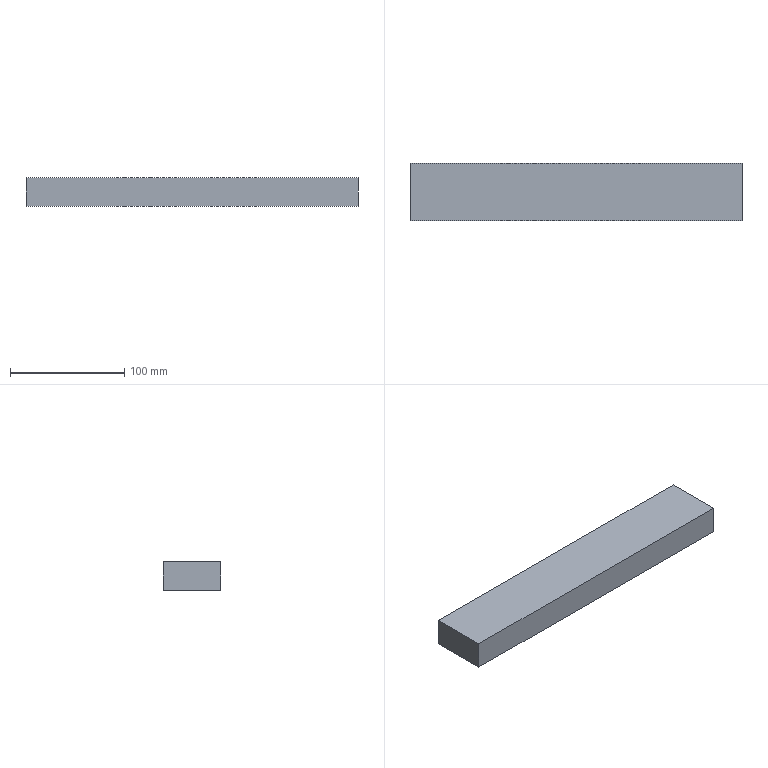Part | SolidWorks | features BaseBody 1 | 1 solid | 6 faces | box 290 x 50 x 25 mm | volume 362500 mm3 | plane 6
STEP:
#1=CARTESIAN_POINT('',(-145.,25.,0.));
#2=VERTEX_POINT('',#1);
#3=CARTESIAN_POINT('',(-145.,-25.,0.));
#4=VERTEX_POINT('',#3);
#5=CARTESIAN_POINT('',(-145.,-25.,0.));
#6=DIRECTION('',(0.,-1.,0.));
#7=VECTOR('',#6,1000.);
#8=LINE('',#5,#7);
#9=EDGE_CURVE('',#2,#4,#8,.T.);
#10=ORIENTED_EDGE('',*,*,#9,.T.);
#11=CARTESIAN_POINT('',(-145.,-25.,25.));
#12=VERTEX_POINT('',#11);
#13=CARTESIAN_POINT('',(-145.,-25.,25.));
#14=DIRECTION('',(0.,0.,-1.));
#15=VECTOR('',#14,1000.);
#16=LINE('',#13,#15);
#17=EDGE_CURVE('',#12,#4,#16,.T.);
#18=ORIENTED_EDGE('',*,*,#17,.F.);
#19=CARTESIAN_POINT('',(-145.,25.,25.));
#20=VERTEX_POINT('',#19);
#21=CARTESIAN_POINT('',(-145.,-25.,25.));
#22=DIRECTION('',(0.,-1.,0.));
#23=VECTOR('',#22,1000.);
#24=LINE('',#21,#23);
#25=EDGE_CURVE('',#20,#12,#24,.T.);
#26=ORIENTED_EDGE('',*,*,#25,.F.);
#27=CARTESIAN_POINT('',(-145.,25.,25.));
#28=DIRECTION('',(0.,0.,-1.));
#29=VECTOR('',#28,1000.);
#30=LINE('',#27,#29);
#31=EDGE_CURVE('',#20,#2,#30,.T.);
#32=ORIENTED_EDGE('',*,*,#31,.T.);
#33=EDGE_LOOP('',(#10,#18,#26,#32));
#34=FACE_OUTER_BOUND('',#33,.T.);
#35=CARTESIAN_POINT('',(-145.,-25.,25.));
#36=DIRECTION('',(1.,0.,0.));
#37=DIRECTION('',(0.,0.,-1.));
#38=AXIS2_PLACEMENT_3D('',#35,#36,#37);
#39=PLANE('',#38);
#40=ADVANCED_FACE('',(#34),#39,.F.);
#41=CARTESIAN_POINT('',(145.,-25.,0.));
#42=VERTEX_POINT('',#41);
#43=CARTESIAN_POINT('',(145.,-25.,0.));
#44=DIRECTION('',(1.,0.,0.));
#45=VECTOR('',#44,1000.);
#46=LINE('',#43,#45);
#47=EDGE_CURVE('',#4,#42,#46,.T.);
#48=ORIENTED_EDGE('',*,*,#47,.T.);
#49=CARTESIAN_POINT('',(145.,-25.,25.));
#50=VERTEX_POINT('',#49);
#51=CARTESIAN_POINT('',(145.,-25.,25.));
#52=DIRECTION('',(0.,0.,-1.));
#53=VECTOR('',#52,1000.);
#54=LINE('',#51,#53);
#55=EDGE_CURVE('',#50,#42,#54,.T.);
#56=ORIENTED_EDGE('',*,*,#55,.F.);
#57=CARTESIAN_POINT('',(145.,-25.,25.));
#58=DIRECTION('',(1.,0.,0.));
#59=VECTOR('',#58,1000.);
#60=LINE('',#57,#59);
#61=EDGE_CURVE('',#12,#50,#60,.T.);
#62=ORIENTED_EDGE('',*,*,#61,.F.);
#63=ORIENTED_EDGE('',*,*,#17,.T.);
#64=EDGE_LOOP('',(#48,#56,#62,#63));
#65=FACE_OUTER_BOUND('',#64,.T.);
#66=CARTESIAN_POINT('',(145.,-25.,25.));
#67=DIRECTION('',(0.,1.,0.));
#68=DIRECTION('',(-1.,0.,0.));
#69=AXIS2_PLACEMENT_3D('',#66,#67,#68);
#70=PLANE('',#69);
#71=ADVANCED_FACE('',(#65),#70,.F.);
#72=CARTESIAN_POINT('',(145.,25.,0.));
#73=VERTEX_POINT('',#72);
#74=CARTESIAN_POINT('',(145.,-25.,0.));
#75=DIRECTION('',(0.,1.,0.));
#76=VECTOR('',#75,1000.);
#77=LINE('',#74,#76);
#78=EDGE_CURVE('',#42,#73,#77,.T.);
#79=ORIENTED_EDGE('',*,*,#78,.T.);
#80=CARTESIAN_POINT('',(145.,25.,25.));
#81=VERTEX_POINT('',#80);
#82=CARTESIAN_POINT('',(145.,25.,25.));
#83=DIRECTION('',(0.,0.,-1.));
#84=VECTOR('',#83,1000.);
#85=LINE('',#82,#84);
#86=EDGE_CURVE('',#81,#73,#85,.T.);
#87=ORIENTED_EDGE('',*,*,#86,.F.);
#88=CARTESIAN_POINT('',(145.,-25.,25.));
#89=DIRECTION('',(0.,1.,0.));
#90=VECTOR('',#89,1000.);
#91=LINE('',#88,#90);
#92=EDGE_CURVE('',#50,#81,#91,.T.);
#93=ORIENTED_EDGE('',*,*,#92,.F.);
#94=ORIENTED_EDGE('',*,*,#55,.T.);
#95=EDGE_LOOP('',(#79,#87,#93,#94));
#96=FACE_OUTER_BOUND('',#95,.T.);
#97=CARTESIAN_POINT('',(145.,-25.,25.));
#98=DIRECTION('',(-1.,0.,0.));
#99=DIRECTION('',(0.,0.,1.));
#100=AXIS2_PLACEMENT_3D('',#97,#98,#99);
#101=PLANE('',#100);
#102=ADVANCED_FACE('',(#96),#101,.F.);
#103=CARTESIAN_POINT('',(145.,25.,0.));
#104=DIRECTION('',(-1.,0.,0.));
#105=VECTOR('',#104,1000.);
#106=LINE('',#103,#105);
#107=EDGE_CURVE('',#73,#2,#106,.T.);
#108=ORIENTED_EDGE('',*,*,#107,.T.);
#109=ORIENTED_EDGE('',*,*,#31,.F.);
#110=CARTESIAN_POINT('',(145.,25.,25.));
#111=DIRECTION('',(-1.,0.,0.));
#112=VECTOR('',#111,1000.);
#113=LINE('',#110,#112);
#114=EDGE_CURVE('',#81,#20,#113,.T.);
#115=ORIENTED_EDGE('',*,*,#114,.F.);
#116=ORIENTED_EDGE('',*,*,#86,.T.);
#117=EDGE_LOOP('',(#108,#109,#115,#116));
#118=FACE_OUTER_BOUND('',#117,.T.);
#119=CARTESIAN_POINT('',(145.,25.,25.));
#120=DIRECTION('',(0.,-1.,0.));
#121=DIRECTION('',(1.,0.,0.));
#122=AXIS2_PLACEMENT_3D('',#119,#120,#121);
#123=PLANE('',#122);
#124=ADVANCED_FACE('',(#118),#123,.F.);
#125=ORIENTED_EDGE('',*,*,#25,.T.);
#126=ORIENTED_EDGE('',*,*,#61,.T.);
#127=ORIENTED_EDGE('',*,*,#92,.T.);
#128=ORIENTED_EDGE('',*,*,#114,.T.);
#129=EDGE_LOOP('',(#125,#126,#127,#128));
#130=FACE_OUTER_BOUND('',#129,.T.);
#131=CARTESIAN_POINT('',(0.,0.,25.));
#132=DIRECTION('',(0.,0.,1.));
#133=DIRECTION('',(1.,0.,0.));
#134=AXIS2_PLACEMENT_3D('',#131,#132,#133);
#135=PLANE('',#134);
#136=ADVANCED_FACE('',(#130),#135,.T.);
#137=ORIENTED_EDGE('',*,*,#9,.F.);
#138=ORIENTED_EDGE('',*,*,#107,.F.);
#139=ORIENTED_EDGE('',*,*,#78,.F.);
#140=ORIENTED_EDGE('',*,*,#47,.F.);
#141=EDGE_LOOP('',(#137,#138,#139,#140));
#142=FACE_OUTER_BOUND('',#141,.T.);
#143=CARTESIAN_POINT('',(0.,0.,0.));
#144=DIRECTION('',(0.,0.,1.));
#145=DIRECTION('',(1.,0.,0.));
#146=AXIS2_PLACEMENT_3D('',#143,#144,#145);
#147=PLANE('',#146);
#148=ADVANCED_FACE('',(#142),#147,.F.);
#149=CLOSED_SHELL('',(#40,#71,#102,#124,#136,#148));
#150=MANIFOLD_SOLID_BREP('',#149);
#151=CARTESIAN_POINT('',(0.,0.,0.));
#152=DIRECTION('',(0.,0.,1.));
#153=DIRECTION('',(1.,0.,0.));
#154=AXIS2_PLACEMENT_3D('',#151,#152,#153);
#155=(LENGTH_UNIT()NAMED_UNIT(*)SI_UNIT(.MILLI.,.METRE.));
#156=UNCERTAINTY_MEASURE_WITH_UNIT(LENGTH_MEASURE(0.00001),#155,'','');
#157=(NAMED_UNIT(*)PLANE_ANGLE_UNIT()SI_UNIT($,.RADIAN.));
#158=(NAMED_UNIT(*)SI_UNIT($,.STERADIAN.)SOLID_ANGLE_UNIT());
#159=(GEOMETRIC_REPRESENTATION_CONTEXT(3)GLOBAL_UNCERTAINTY_ASSIGNED_CONTEXT((#156))GLOBAL_UNIT_ASSIGNED_CONTEXT((#155,#157,#158))REPRESENTATION_CONTEXT('',''));
#160=ADVANCED_BREP_SHAPE_REPRESENTATION('',(#150,#154),#159);